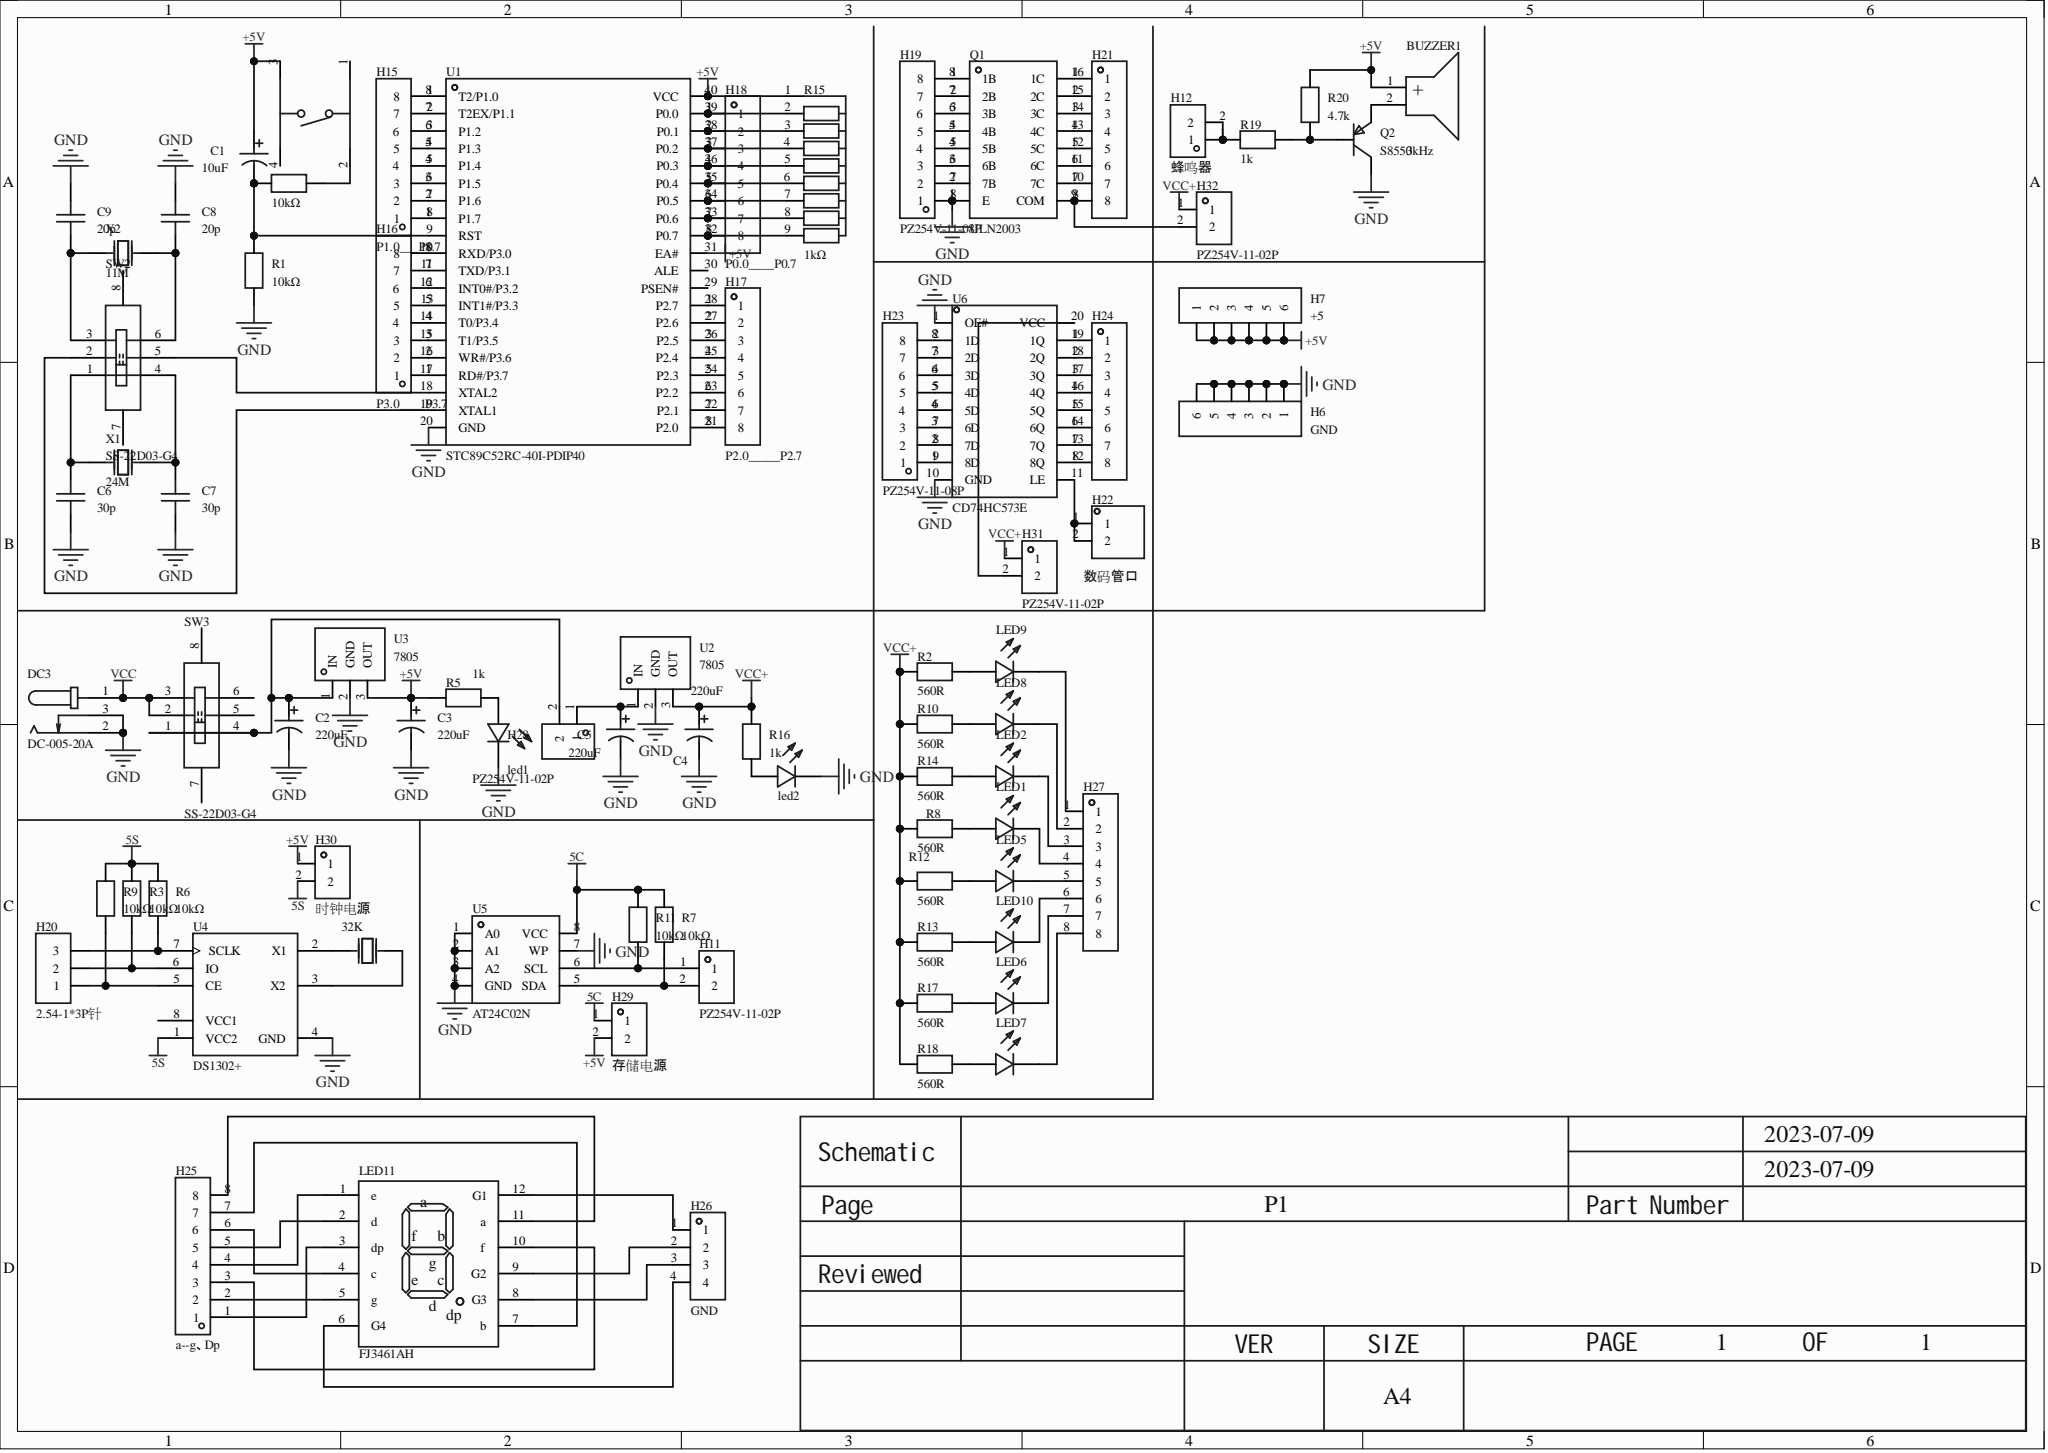Circuit board | Altium Designer | 78 parts | 121 nets
Bill of materials:
Comment,Description,Designator,Footprint,LibRef,Quantity
"3kHz","","BUZZER1","BUZ-TH_BD9.0-P5.00-D0.6-FD","HNB09A03","1"
"10uF","","C1","CAP-TH_BD5.0-P2.00-D0.8-FD","ERS1HM100D11OT","1"
"220uF","","C2, C3, C4, C5","CAP-TH_BD8.0-P3.50-D0.6-FD","KM227M035F12RR0VH2FP0","4"
"30p","","C6, C7","CAP-TH_L5.0-W5.0-P2.54-D1.0","CC1H150KA1FDCH4B1000","2"
"20p","","C8, C9","CAP-TH_L5.0-W5.0-P2.54-D1.0","CC1H150KA1FDCH4B1000","2"
"DC-005-20A","","DC3","DC-IN-TH_DC-005-20A","DC-005-20A_C136744","1"
"GND","","H6","HDR-TH_6P-P2.54-V-M-1","2.54-1x6P直针","1"
"+5","","H7","HDR-TH_6P-P2.54-V-M-1","2.54-1x6P直针","1"
"PZ254V-11-02P","","H11, H28, H31, H32","HDR-TH_2P-P2.54-V-M","PZ254V-11-02P","4"
"蜂鸣器","","H12","HDR-TH_2P-P2.54-V-M","PZ254V-11-02P","1"
"P1.0___P1.7","","H15","HDR-TH_8P-P2.54-V-M","PZ254V-11-08P","1"
"P3.0____P3.7","","H16","HDR-TH_8P-P2.54-V-M","PZ254V-11-08P","1"
"P2.0_____P2.7","","H17","HDR-TH_8P-P2.54-V-M","PZ254V-11-08P","1"
"P0.0____P0.7","","H18","HDR-TH_8P-P2.54-V-M","PZ254V-11-08P","1"
"PZ254V-11-08P","","H19, H21, H23, H24, H27","HDR-TH_8P-P2.54-V-M","PZ254V-11-08P","5"
"2.54-1*3P针","","H20","HDR-TH_3P-P2.54-V-M-1","2.54-1*3P针","1"
"数码管口","","H22","HDR-TH_2P-P2.54-V-M-1","B-2100S02P-A110","1"
"a--g、Dp","","H25","HDR-TH_8P-P2.54-V-M","PZ254V-11-08P","1"
"GND","","H26","HDR-TH_4P-P2.54-V-M","PZ254V-11-04P","1"
"存储电源","","H29","HDR-TH_2P-P2.54-V-M","PZ254V-11-02P","1"
"时钟电源","","H30","HDR-TH_2P-P2.54-V-M","PZ254V-11-02P","1"
"204-10SURD/S530-A3-L","","LED1, LED2, LED5, LED6, LED7, LED8, LED9, LED10","LED-TH_BD3.0-P2.54-FD","204-10SURD/S530-A3-L","8"
"led1","","LED3","LED-TH_BD3.0-P2.54-FD","204-10SURD/S530-A3-L","1"
"led2","","LED4","LED-TH_BD3.0-P2.54-FD","204-10SURD/S530-A3-L","1"
"FJ3461AH","","LED11","LED-SEG-TH_12P-L30.0-W14.0-P2.54-S10.16-BL","FJ3461AH","1"
"ULN2003","","Q1","DIP-16_L19.8-W6.5-P2.54-LS7.6-BL","ULN2003_C557872","1"
"S8550","","Q2","TO-92-3_L4.9-W3.7-P1.27-L","S8550_C717454","1"
"10kΩ","","R1, R3, R4, R6, R7, R9, R11","RES-TH_BD2.4-L6.3-P10.30-D0.6","RN1/4W10KFT/BA1","7"
"560R","","R2, R8, R10, R12, R13, R14, R17, R18","RES-TH_BD2.4-L6.3-P10.30-D0.6","RN1/4W10KFT/BA1","8"
"1k","","R5, R16, R19","RES-TH_BD2.4-L6.3-P10.30-D0.6","RN1/4W10KFT/BA1","3"
"1kΩ","","R15","RES-ARRAY-TH_9P-L22.8-W3.00-P2.54","4609X-101-102LF","1"
"4.7k","","R20","RES-TH_BD2.4-L6.3-P10.30-D0.6","RN1/4W10KFT/BA1","1"
"TS-1095-A7B2-D1","","SW1","SW-TH_4P-L6.0-W6.0-P4.50-LS6.5","TS-1095-A7B2-D1","1"
"SS-22D03-G4","","SW2, SW3","SW-TH_SS-22D03-G4","SS-22D03-G4_C136717","2"
"STC89C52RC-40I-PDIP40","","U1","DIP-40_L52.0-W13.7-P2.54-LS15.2-BL","STC89C52RC-40I-PDIP40","1"
"7805","","U2, U3","TO-220-3_L10.0-W4.5-P2.54-L","7805_C2843718","2"
"DS1302+","","U4","DIP-8_L9.8-W6.6-P2.54-LS7.6-BL","DS1302+","1"
"AT24C02N","","U5","DIP-8_L9.2-W6.3-P2.54-LS7.62-BL","AT24C02N","1"
"CD74HC573E","","U6","DIP-20_L26.8-W6.4-P2.54-LS7.6-BL","CD74HC573E","1"
"24M","","X1","HC-49US_L11.5-W4.5-P4.88","X49SD12MSD2SC","1"
"11M","","X2","HC-49US_L11.5-W4.5-P4.88","X49SD12MSD2SC","1"
"32K","","X3","HC-49US_L11.5-W4.5-P4.88","X49SD12MSD2SC","1"
Netlist (Protel format):
[
BUZZER1
BUZ-TH_BD9.0-P5.00-D0.6-FD
3kHz



]
[
C1
CAP-TH_BD5.0-P2.00-D0.8-FD
10uF



]
[
C2
CAP-TH_BD8.0-P3.50-D0.6-FD
220uF



]
[
C3
CAP-TH_BD8.0-P3.50-D0.6-FD
220uF



]
[
C4
CAP-TH_BD8.0-P3.50-D0.6-FD
220uF



]
[
C5
CAP-TH_BD8.0-P3.50-D0.6-FD
220uF



]
[
C6
CAP-TH_L5.0-W5.0-P2.54-D1.0
30p



]
[
C7
CAP-TH_L5.0-W5.0-P2.54-D1.0
30p



]
[
C8
CAP-TH_L5.0-W5.0-P2.54-D1.0
20p



]
[
C9
CAP-TH_L5.0-W5.0-P2.54-D1.0
20p



]
[
DC3
DC-IN-TH_DC-005-20A
DC-005-20A



]
[
H6
HDR-TH_6P-P2.54-V-M-1
GND



]
[
H7
HDR-TH_6P-P2.54-V-M-1
+5



]
[
H11
HDR-TH_2P-P2.54-V-M
PZ254V-11-02P



]
[
H12
HDR-TH_2P-P2.54-V-M
蜂鸣器



]
[
H15
HDR-TH_8P-P2.54-V-M
P1.0___P1.7



]
[
H16
HDR-TH_8P-P2.54-V-M
P3.0____P3.7



]
[
H17
HDR-TH_8P-P2.54-V-M
P2.0_____P2.7



]
[
H18
HDR-TH_8P-P2.54-V-M
P0.0____P0.7



]
[
H19
HDR-TH_8P-P2.54-V-M
PZ254V-11-08P



]
[
H20
HDR-TH_3P-P2.54-V-M-1
2.54-1*3P针



]
[
H21
HDR-TH_8P-P2.54-V-M
PZ254V-11-08P



]
[
H22
HDR-TH_2P-P2.54-V-M-1
数码管口



]
[
H23
HDR-TH_8P-P2.54-V-M
PZ254V-11-08P



]
[
H24
HDR-TH_8P-P2.54-V-M
PZ254V-11-08P



]
[
H25
HDR-TH_8P-P2.54-V-M
a--g、Dp



]
[
H26
HDR-TH_4P-P2.54-V-M
GND



]
[
H27
HDR-TH_8P-P2.54-V-M
PZ254V-11-08P



]
[
H28
HDR-TH_2P-P2.54-V-M
PZ254V-11-02P



]
[
H29
HDR-TH_2P-P2.54-V-M
存储电源



]
[
H30
HDR-TH_2P-P2.54-V-M
时钟电源



]
[
H31
HDR-TH_2P-P2.54-V-M
PZ254V-11-02P



]
[
H32
HDR-TH_2P-P2.54-V-M
PZ254V-11-02P



]
[
LED1
LED-TH_BD3.0-P2.54-FD
204-10SURD/S530-A3-L



]
[
LED2
LED-TH_BD3.0-P2.54-FD
204-10SURD/S530-A3-L



]
[
LED3
LED-TH_BD3.0-P2.54-FD
led1



]
[
LED4
LED-TH_BD3.0-P2.54-FD
led2



]
[
LED5
LED-TH_BD3.0-P2.54-FD
204-10SURD/S530-A3-L



]
[
LED6
LED-TH_BD3.0-P2.54-FD
204-10SURD/S530-A3-L



]
[
LED7
LED-TH_BD3.0-P2.54-FD
204-10SURD/S530-A3-L



]
[
LED8
LED-TH_BD3.0-P2.54-FD
204-10SURD/S530-A3-L



]
[
LED9
LED-TH_BD3.0-P2.54-FD
204-10SURD/S530-A3-L



]
[
LED10
LED-TH_BD3.0-P2.54-FD
204-10SURD/S530-A3-L



]
[
LED11
LED-SEG-TH_12P-L30.0-W14.0-P2.54-S10.16-BL
FJ3461AH



]
[
Q1
DIP-16_L19.8-W6.5-P2.54-LS7.6-BL
ULN2003



]
[
Q2
TO-92-3_L4.9-W3.7-P1.27-L
S8550



]
[
R1
RES-TH_BD2.4-L6.3-P10.30-D0.6
10kΩ



]
[
R2
RES-TH_BD2.4-L6.3-P10.30-D0.6
560R



]
[
R3
RES-TH_BD2.4-L6.3-P10.30-D0.6
10kΩ



]
[
R4
RES-TH_BD2.4-L6.3-P10.30-D0.6
10kΩ



]
[
R5
RES-TH_BD2.4-L6.3-P10.30-D0.6
1k



]
[
R6
RES-TH_BD2.4-L6.3-P10.30-D0.6
10kΩ



]
[
R7
RES-TH_BD2.4-L6.3-P10.30-D0.6
10kΩ



]
[
R8
RES-TH_BD2.4-L6.3-P10.30-D0.6
560R



]
[
R9
RES-TH_BD2.4-L6.3-P10.30-D0.6
10kΩ



]
[
R10
RES-TH_BD2.4-L6.3-P10.30-D0.6
560R



]
[
R11
RES-TH_BD2.4-L6.3-P10.30-D0.6
10kΩ



]
[
R12
RES-TH_BD2.4-L6.3-P10.30-D0.6
560R



]
[
R13
RES-TH_BD2.4-L6.3-P10.30-D0.6
560R



]
[
R14
RES-TH_BD2.4-L6.3-P10.30-D0.6
560R



]
[
R15
RES-ARRAY-TH_9P-L22.8-W3.00-P2.54
1kΩ



]
[
R16
RES-TH_BD2.4-L6.3-P10.30-D0.6
1k



]
[
R17
RES-TH_BD2.4-L6.3-P10.30-D0.6
560R



]
[
R18
RES-TH_BD2.4-L6.3-P10.30-D0.6
560R



]
[
R19
RES-TH_BD2.4-L6.3-P10.30-D0.6
1k



]
[
R20
RES-TH_BD2.4-L6.3-P10.30-D0.6
4.7k



]
[
SW1
SW-TH_4P-L6.0-W6.0-P4.50-LS6.5
TS-1095-A7B2-D1



]
[
SW2
SW-TH_SS-22D03-G4
SS-22D03-G4



]
[
SW3
SW-TH_SS-22D03-G4
SS-22D03-G4



]
[
U1
DIP-40_L52.0-W13.7-P2.54-LS15.2-BL
STC89C52RC-40I-PDIP40



]
[
U2
TO-220-3_L10.0-W4.5-P2.54-L
7805



]
[
U3
TO-220-3_L10.0-W4.5-P2.54-L
7805



]
[
U4
DIP-8_L9.8-W6.6-P2.54-LS7.6-BL
DS1302+



]
[
U5
DIP-8_L9.2-W6.3-P2.54-LS7.62-BL
AT24C02N



]
[
U6
DIP-20_L26.8-W6.4-P2.54-LS7.6-BL
CD74HC573E



]
[
X1
HC-49US_L11.5-W4.5-P4.88
24M



]
[
X2
HC-49US_L11.5-W4.5-P4.88
11M



]
[
X3
HC-49US_L11.5-W4.5-P4.88
32K



]
(
VCC+
C4-1
H31-1
H32-1
R2-1
R8-1
R10-1
R12-1
R13-1
R14-1
R16-2
R17-1
R18-1
U2-3
)
(
VCC
DC3-1
SW3-2
SW3-3
)
(
NetU4_3
U4-3
X3-1
)
(
NetU4_2
U4-2
X3-2
)
(
NetSW2_5
SW2-5
U1-18
)
(
NetSW2_2
SW2-2
U1-19
)
(
NetR4_2
R4-2
SW1-2
)
(
NetQ2_2
Q2-2
R19-2
R20-1
)
(
NetLED10_1
LED10-1
R13-2
)
(
NetLED9_1
LED9-1
R2-2
)
(
NetLED8_1
LED8-1
R10-2
)
(
NetLED7_1
LED7-1
R18-2
)
(
NetLED6_1
LED6-1
R17-2
)
(
NetLED5_1
LED5-1
R12-2
)
(
NetLED4_1
LED4-1
R16-1
)
(
NetLED3_1
LED3-1
R5-2
)
(
NetLED2_1
LED2-1
R14-2
)
(
NetLED1_1
LED1-1
R8-2
)
(
NetH31_2
H31-2
U6-20
)
(
NetH27_8
H27-8
LED7-2
)
(
NetH27_7
H27-7
LED6-2
)
(
NetH27_6
H27-6
LED10-2
)
(
NetH27_5
H27-5
LED5-2
)
(
NetH27_4
H27-4
LED1-2
)
(
NetH27_3
H27-3
LED2-2
)
(
NetH27_2
H27-2
LED8-2
)
(
NetH27_1
H27-1
LED9-2
)
(
NetH26_4
H26-4
LED11-6
)
(
NetH26_3
H26-3
LED11-8
)
(
NetH26_2
H26-2
LED11-9
)
(
NetH26_1
H26-1
LED11-12
)
(
NetH25_8
H25-8
LED11-11
)
(
NetH25_7
H25-7
LED11-7
)
(
NetH25_6
H25-6
LED11-4
)
(
NetH25_5
H25-5
LED11-2
)
(
NetH25_4
H25-4
LED11-1
)
(
NetH25_3
H25-3
LED11-10
)
(
NetH25_2
H25-2
LED11-5
)
(
NetH25_1
H25-1
LED11-3
)
(
NetH24_8
H24-8
U6-12
)
(
NetH24_7
H24-7
U6-13
)
(
NetH24_6
H24-6
U6-14
)
(
NetH24_5
H24-5
U6-15
)
(
NetH24_4
H24-4
U6-16
)
(
NetH24_3
H24-3
U6-17
)
(
NetH24_2
H24-2
U6-18
)
(
NetH24_1
H24-1
U6-19
)
(
NetH23_8
H23-8
U6-2
)
(
NetH23_7
H23-7
U6-3
)
(
NetH23_6
H23-6
U6-4
)
(
NetH23_5
H23-5
U6-5
)
(
NetH23_4
H23-4
U6-6
)
(
NetH23_3
H23-3
U6-7
)
(
NetH23_2
H23-2
U6-8
)
(
NetH23_1
H23-1
U6-9
)
(
NetH22_1
H22-1
H22-2
U6-11
)
(
NetH21_8
H21-8
H32-2
Q1-9
)
(
NetH21_7
H21-7
Q1-10
)
(
NetH21_6
H21-6
Q1-11
)
(
NetH21_5
H21-5
Q1-12
)
(
NetH21_4
H21-4
Q1-13
)
(
NetH21_3
H21-3
Q1-14
)
(
NetH21_2
H21-2
Q1-15
)
(
NetH21_1
H21-1
Q1-16
)
(
NetH20_3
H20-3
R6-1
U4-7
)
(
NetH20_2
H20-2
R3-1
U4-6
)
(
NetH20_1
H20-1
R9-1
U4-5
)
(
NetH19_8
H19-8
Q1-1
)
(
NetH19_7
H19-7
Q1-2
)
(
NetH19_6
H19-6
Q1-3
)
(
NetH19_5
H19-5
Q1-4
)
(
NetH19_4
H19-4
Q1-5
)
(
NetH19_3
H19-3
Q1-6
)
(
NetH19_2
H19-2
Q1-7
)
(
NetH18_8
H18-8
R15-9
U1-32
)
(
NetH18_7
H18-7
R15-8
U1-33
)
(
NetH18_6
H18-6
R15-7
U1-34
)
(
NetH18_5
H18-5
R15-6
U1-35
)
(
NetH18_4
H18-4
R15-5
U1-36
)
(
NetH18_3
H18-3
R15-4
U1-37
)
(
NetH18_2
H18-2
R15-3
U1-38
)
(
NetH18_1
H18-1
R15-2
U1-39
)
(
NetH17_8
H17-8
U1-21
)
(
NetH17_7
H17-7
U1-22
)
(
NetH17_6
H17-6
U1-23
)
(
NetH17_5
H17-5
U1-24
)
(
NetH17_4
H17-4
U1-25
)
(
NetH17_3
H17-3
U1-26
)
(
NetH17_2
H17-2
U1-27
)
(
NetH17_1
H17-1
U1-28
)
(
NetH16_8
H16-8
U1-10
)
(
NetH16_7
H16-7
U1-11
)
(
NetH16_6
H16-6
U1-12
)
(
NetH16_5
H16-5
U1-13
)
(
NetH16_4
H16-4
U1-14
)
(
NetH16_3
H16-3
U1-15
)
(
NetH16_2
H16-2
U1-16
)
(
NetH16_1
H16-1
U1-17
)
(
NetH15_8
H15-8
U1-1
)
(
NetH15_7
H15-7
U1-2
)
(
NetH15_6
H15-6
U1-3
)
(
NetH15_5
H15-5
U1-4
)
(
NetH15_4
H15-4
U1-5
)
(
NetH15_3
H15-3
U1-6
)
(
NetH15_2
H15-2
U1-7
)
(
NetH15_1
H15-1
U1-8
)
(
NetH12_1
H12-1
H12-2
R19-1
)
(
NetH11_2
H11-2
R7-1
U5-5
)
(
NetH11_1
H11-1
R11-1
U5-6
)
(
NetC9_2
C9-2
SW2-3
X2-1
)
(
NetC8_1
C8-1
SW2-6
X2-2
)
(
NetC7_2
C7-2
SW2-4
X1-1
)
(
NetC6_2
C6-2
SW2-1
X1-2
)
(
NetC5_1
C5-1
H28-1
U2-1
)
(
NetC2_1
C2-1
H28-2
SW3-1
SW3-4
U3-1
)
(
NetC1_2
C1-2
R1-2
R4-1
U1-9
)
(
NetBUZZER1_2
BUZZER1-2
Q2-1
)
(
GND
C2-2
C3-2
C4-2
C5-2
C6-1
C7-1
C8-2
C9-1
DC3-2
DC3-3
H6-1
H6-2
H6-3
H6-4
H6-5
H6-6
H19-1
LED3-2
LED4-2
Q1-8
Q2-3
R1-1
U1-20
U2-2
U3-2
U4-4
U5-1
U5-2
U5-3
U5-4
U5-7
U6-1
U6-10
)
(
+5V
BUZZER1-1
C1-1
C3-1
H7-1
H7-2
H7-3
H7-4
H7-5
H7-6
H29-2
H30-1
R5-1
R15-1
R20-2
SW1-3
U1-31
U1-40
U3-3
)
(
5S
H30-2
R3-2
R6-2
R9-2
U4-1
)
(
5C
H29-1
R7-2
R11-2
U5-8
)